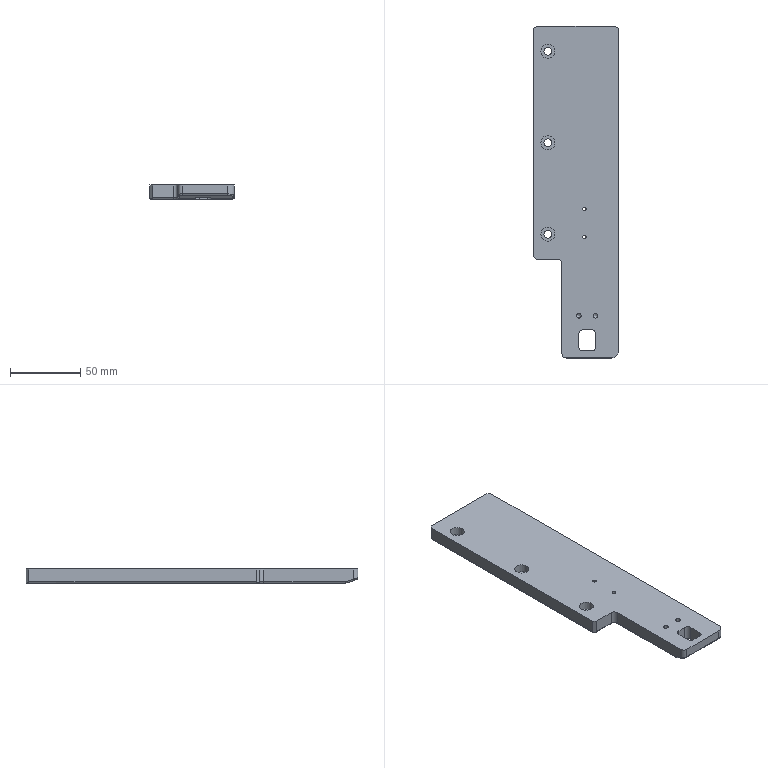NC program | NX | posted with a generic post | part box 60 x 236 x 10 mm
Whole program:
N10 G17 G21 G94 G90
(FLOOR_WALL_COPY , TOOL : D80)
N12 T19 M6
N14 G54
N16 G17 G0 G90 X279. Y-30. S6500 M3
N18 G43 Z30. H19
N20 Z3.
N22 G94 G1 Z0. F1500.
N24 X276.
N26 X-40.
N28 X-43.
N30 Z3.
N32 G0 Z30.
N34 M5
(DRILLING_COPY , TOOL : D6A45)
N36 T01 M6
N38 G54
N40 G17 G0 G90 X206. Y-16. S9500 M3
N42 G43 Z30. H1
N44 G94 G81 G98 Z-1.8 F250. R3.
N46 Y-28.
N48 G80
N50 G0 X206. Y-28. Z30.
N52 M5
(HOLE_MILLING , TOOL : D6)
N54 T12 M6
N56 G54
N58 G17 G0 G90 X18. Y-50. S9500 M3
N60 G43 Z30. H12
N62 Z0.5
N64 G94 G3 X19. Y-49. R1. F1450.
N66 X18. Y-48. R1.
N68 X18. Y-48. Z-0.1 I0. J-2.
N70 X18. Y-48. Z-0.7 I0. J-2.
N72 X18. Y-48. Z-1.3 I0. J-2.
N74 X18. Y-48. Z-1.9 I0. J-2.
N76 X18. Y-48. Z-2.5 I0. J-2.
N78 X18. Y-48. Z-3.1 I0. J-2.
N80 X18. Y-48. Z-3.7 I0. J-2.
N82 X18. Y-48. Z-4.3 I0. J-2.
N84 X18. Y-48. Z-4.9 I0. J-2.
N86 X18. Y-48. Z-5.5 I0. J-2.
N88 X19.732 Y-49. Z-6. R-2.
N90 X17. Y-48.268 R2.
N92 X19.732 Y-49. R-2.
N94 X18.366 Y-48.634 R1.
N96 X18. Y-50. R1.
N98 G0 Z30.
N100 X83.
N102 Z0.5
N104 G3 X84. Y-49. R1.
N106 X83. Y-48. R1.
N108 X83. Y-48. Z-0.1 I0. J-2.
N110 X83. Y-48. Z-0.7 I0. J-2.
N112 X83. Y-48. Z-1.3 I0. J-2.
N114 X83. Y-48. Z-1.9 I0. J-2.
N116 X83. Y-48. Z-2.5 I0. J-2.
N118 X83. Y-48. Z-3.1 I0. J-2.
N120 X83. Y-48. Z-3.7 I0. J-2.
N122 X83. Y-48. Z-4.3 I0. J-2.
N124 X83. Y-48. Z-4.9 I0. J-2.
N126 X83. Y-48. Z-5.5 I0. J-2.
N128 X84.732 Y-49. Z-6. R-2.
N130 X82. Y-48.268 R2.
N132 X84.732 Y-49. R-2.
N134 X83.366 Y-48.634 R1.
N136 X83. Y-50. R1.
N138 G0 Z30.
N140 X148.
N142 Z0.5
N144 G3 X149. Y-49. R1.
N146 X148. Y-48. R1.
N148 X148. Y-48. Z-0.1 I0. J-2.
N150 X148. Y-48. Z-0.7 I0. J-2.
N152 X148. Y-48. Z-1.3 I0. J-2.
N154 X148. Y-48. Z-1.9 I0. J-2.
N156 X148. Y-48. Z-2.5 I0. J-2.
N158 X148. Y-48. Z-3.1 I0. J-2.
N160 X148. Y-48. Z-3.7 I0. J-2.
N162 X148. Y-48. Z-4.3 I0. J-2.
N164 X148. Y-48. Z-4.9 I0. J-2.
N166 X148. Y-48. Z-5.5 I0. J-2.
N168 X149.732 Y-49. Z-6. R-2.
N170 X147. Y-48.268 R2.
N172 X149.732 Y-49. R-2.
N174 X148.366 Y-48.634 R1.
N176 X148. Y-50. R1.
N178 G0 Z30.
N180 M5
(DRILLING_COPY_COPY_COPY_1 , TOOL : 3.2ZT)
N182 T03 M6
N184 G54
N186 G17 G0 G90 X206. Y-28. S2000 M3
N188 G43 Z30. H3
N190 G94 G83 G98 Z-8.974 F150. Q2. R3.
N192 Y-16.
N194 G80
N196 G0 X206. Y-16. Z30.
N198 M5
(PLANAR_MILL_COPY_COPY , TOOL : D6A45)
N200 T01 M6
N202 G54
N204 G17 G0 G90 X17.134 Y-53.6 S9500 M3
N206 G43 Z30. H1
N208 Z0.5
N210 G94 G1 Z-1. F1250.
N212 G3 X18. Y-54.1 R1.
N214 X22.1 Y-50. R4.1
N216 X18. Y-54.1 R-4.1
N218 X18.866 Y-53.6 R1.
N220 G1 Z0.5
N222 G0 Z30.
N224 X82.134
N226 Z0.5
N228 G1 Z-1.
N230 G3 X83. Y-54.1 R1.
N232 X87.1 Y-50. R4.1
N234 X83. Y-54.1 R-4.1
N236 X83.866 Y-53.6 R1.
N238 G1 Z0.5
N240 G0 Z30.
N242 X115.634 Y1.4
N244 Z0.5
N246 G1 Z-1.
N248 G3 X116.5 Y0.9 R1.
N250 G1 X231.
N252 G2 X236.9 Y-5. R5.9
N254 G1 Y-37.
N256 G2 X233. Y-40.9 R3.9
N258 G1 X169.
N260 G3 X166.9 Y-43. R2.1
N262 G1 Y-58.
N264 G2 X166.636 Y-58.636 R0.9
N266 G1 X164.636 Y-60.636
N268 G2 X164. Y-60.9 R0.9
N270 G1 X2.
N272 G2 X1.364 Y-60.636 R0.9
N274 G1 X-0.636 Y-58.636
N276 G2 X-0.9 Y-58. R0.9
N278 G1 Y-2.
N280 G2 X-0.636 Y-1.364 R0.9
N282 G1 X1.364 Y0.636
N284 G2 X2. Y0.9 R0.9
N286 G1 X116.5
N288 G3 X117.366 Y1.4 R1.
N290 G1 Z0.5
N292 G0 Z30.
N294 X129.742 Y-24.099
N296 Z0.5
N298 G1 Z-1.
N300 G3 X130. Y-23.671 R0.5
N302 X129.671 Y-24. R0.33
N304 X130. Y-23.671 R-0.33
N306 X130.258 Y-24.099 R0.5
N308 G1 Z0.5
N310 G0 Z30.
N312 X147.134 Y-53.6
N314 Z0.5
N316 G1 Z-1.
N318 G3 X148. Y-54.1 R1.
N320 X152.1 Y-50. R4.1
N322 X148. Y-54.1 R-4.1
N324 X148.866 Y-53.6 R1.
N326 G1 Z0.5
N328 G0 Z30.
N330 X149.742 Y-24.099
N332 Z0.5
N334 G1 Z-1.
N336 G3 X150. Y-23.671 R0.5
N338 X149.671 Y-24. R0.33
N340 X150. Y-23.671 R-0.33
N342 X150.258 Y-24.099 R0.5
N344 G1 Z0.5
N346 G0 Z30.
N348 X206.433 Y-27.529
N350 Z0.5
N352 G1 Z-1.
N354 G3 X206. Y-27.279 R0.5
N356 X205.279 Y-28. R0.721
N358 X206. Y-27.279 R-0.721
N360 X205.567 Y-27.529 R0.5
N362 G1 Z0.5
N364 G0 Z30.
N366 X206.433 Y-15.529
N368 Z0.5
N370 G1 Z-1.
N372 G3 X206. Y-15.279 R0.5
N374 X205.279 Y-16. R0.721
N376 X206. Y-15.279 R-0.721
N378 X205.567 Y-15.529 R0.5
N380 G1 Z0.5
N382 G0 Z30.
N384 X224.366 Y-17.4
N386 Z0.5
N388 G1 Z-1.
N390 G3 X223.5 Y-16.9 R1.
N392 G1 X219.
N394 G3 X216.9 Y-19. R2.1
N396 G1 Y-25.
N398 G3 X219. Y-27.1 R2.1
N400 G1 X228.
N402 G3 X230.1 Y-25. R2.1
N404 G1 Y-19.
N406 G3 X228. Y-16.9 R2.1
N408 G1 X223.5
N410 G3 X222.634 Y-17.4 R1.
N412 G1 Z0.5
N414 G0 Z30.
N416 M5
N418 M2